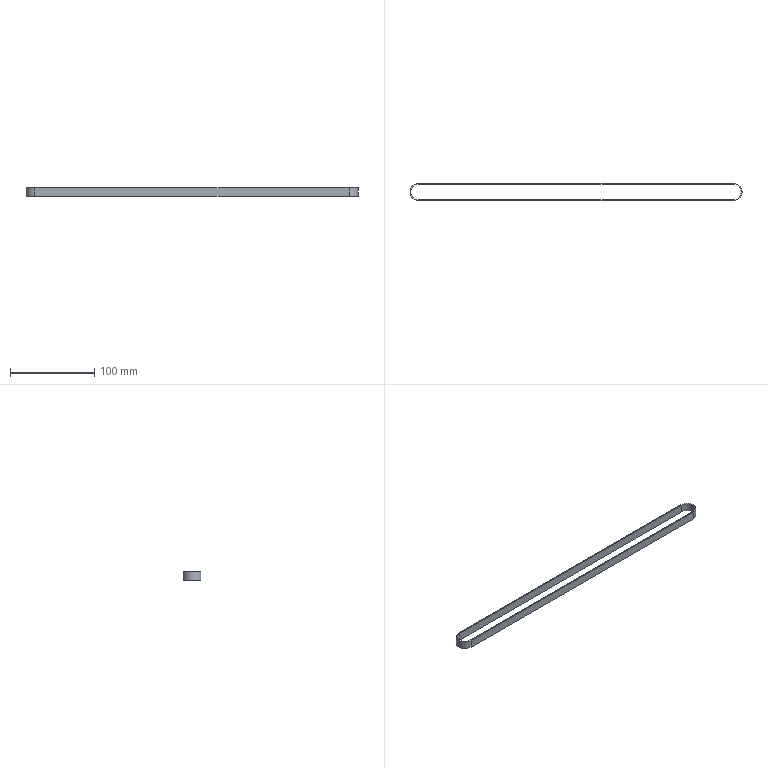Part | SolidWorks | features BaseBody 1 | 1 solid | 12 faces | box 395.01 x 21.01 x 10 mm | volume 8109 mm3 | cylinder 6 | plane 6 | commonest cylinder face diameters 19.01 x3 21.01 x3
STEP:
#1=CARTESIAN_POINT('',(334.,4.505,0.));
#2=VERTEX_POINT('',#1);
#3=CARTESIAN_POINT('',(343.505,-5.,0.));
#4=VERTEX_POINT('',#3);
#5=CARTESIAN_POINT('',(334.,-5.,0.));
#6=DIRECTION('',(0.,0.,-1.));
#7=DIRECTION('',(1.,0.,0.));
#8=AXIS2_PLACEMENT_3D('',#5,#6,#7);
#9=CIRCLE('',#8,9.505);
#10=EDGE_CURVE('',#2,#4,#9,.T.);
#11=ORIENTED_EDGE('',*,*,#10,.T.);
#12=CARTESIAN_POINT('',(343.505,-5.,10.));
#13=VERTEX_POINT('',#12);
#14=CARTESIAN_POINT('',(343.505,-5.,0.));
#15=DIRECTION('',(0.,0.,1.));
#16=VECTOR('',#15,1000.);
#17=LINE('',#14,#16);
#18=EDGE_CURVE('',#4,#13,#17,.T.);
#19=ORIENTED_EDGE('',*,*,#18,.T.);
#20=CARTESIAN_POINT('',(334.,4.505,10.));
#21=VERTEX_POINT('',#20);
#22=CARTESIAN_POINT('',(334.,-5.,10.));
#23=DIRECTION('',(0.,0.,-1.));
#24=DIRECTION('',(1.,0.,0.));
#25=AXIS2_PLACEMENT_3D('',#22,#23,#24);
#26=CIRCLE('',#25,9.505);
#27=EDGE_CURVE('',#21,#13,#26,.T.);
#28=ORIENTED_EDGE('',*,*,#27,.F.);
#29=CARTESIAN_POINT('',(334.,4.505,0.));
#30=DIRECTION('',(0.,0.,-1.));
#31=VECTOR('',#30,1000.);
#32=LINE('',#29,#31);
#33=EDGE_CURVE('',#21,#2,#32,.T.);
#34=ORIENTED_EDGE('',*,*,#33,.T.);
#35=EDGE_LOOP('',(#11,#19,#28,#34));
#36=FACE_OUTER_BOUND('',#35,.T.);
#37=CARTESIAN_POINT('',(334.,-5.,0.));
#38=DIRECTION('',(0.,0.,1.));
#39=DIRECTION('',(1.,0.,0.));
#40=AXIS2_PLACEMENT_3D('',#37,#38,#39);
#41=CYLINDRICAL_SURFACE('',#40,9.505);
#42=ADVANCED_FACE('',(#36),#41,.F.);
#43=CARTESIAN_POINT('',(334.,-15.505,0.));
#44=VERTEX_POINT('',#43);
#45=CARTESIAN_POINT('',(344.505,-5.,0.));
#46=VERTEX_POINT('',#45);
#47=CARTESIAN_POINT('',(334.,-5.,0.));
#48=DIRECTION('',(0.,0.,1.));
#49=DIRECTION('',(1.,0.,0.));
#50=AXIS2_PLACEMENT_3D('',#47,#48,#49);
#51=CIRCLE('',#50,10.505);
#52=EDGE_CURVE('',#44,#46,#51,.T.);
#53=ORIENTED_EDGE('',*,*,#52,.T.);
#54=CARTESIAN_POINT('',(344.505,-5.,10.));
#55=VERTEX_POINT('',#54);
#56=CARTESIAN_POINT('',(344.505,-5.,0.));
#57=DIRECTION('',(0.,0.,1.));
#58=VECTOR('',#57,1000.);
#59=LINE('',#56,#58);
#60=EDGE_CURVE('',#46,#55,#59,.T.);
#61=ORIENTED_EDGE('',*,*,#60,.T.);
#62=CARTESIAN_POINT('',(334.,-15.505,10.));
#63=VERTEX_POINT('',#62);
#64=CARTESIAN_POINT('',(334.,-5.,10.));
#65=DIRECTION('',(0.,0.,1.));
#66=DIRECTION('',(1.,0.,0.));
#67=AXIS2_PLACEMENT_3D('',#64,#65,#66);
#68=CIRCLE('',#67,10.505);
#69=EDGE_CURVE('',#63,#55,#68,.T.);
#70=ORIENTED_EDGE('',*,*,#69,.F.);
#71=CARTESIAN_POINT('',(334.,-15.505,0.));
#72=DIRECTION('',(0.,0.,-1.));
#73=VECTOR('',#72,1000.);
#74=LINE('',#71,#73);
#75=EDGE_CURVE('',#63,#44,#74,.T.);
#76=ORIENTED_EDGE('',*,*,#75,.T.);
#77=EDGE_LOOP('',(#53,#61,#70,#76));
#78=FACE_OUTER_BOUND('',#77,.T.);
#79=CARTESIAN_POINT('',(334.,-5.,0.));
#80=DIRECTION('',(0.,0.,1.));
#81=DIRECTION('',(1.,0.,0.));
#82=AXIS2_PLACEMENT_3D('',#79,#80,#81);
#83=CYLINDRICAL_SURFACE('',#82,10.505);
#84=ADVANCED_FACE('',(#78),#83,.T.);
#85=CARTESIAN_POINT('',(-40.,4.505,0.));
#86=VERTEX_POINT('',#85);
#87=CARTESIAN_POINT('',(-40.,4.505,10.));
#88=VERTEX_POINT('',#87);
#89=CARTESIAN_POINT('',(-40.,4.505,0.));
#90=DIRECTION('',(0.,0.,1.));
#91=VECTOR('',#90,1000.);
#92=LINE('',#89,#91);
#93=EDGE_CURVE('',#86,#88,#92,.T.);
#94=ORIENTED_EDGE('',*,*,#93,.F.);
#95=CARTESIAN_POINT('',(-40.,4.505,0.));
#96=DIRECTION('',(-1.,0.,0.));
#97=VECTOR('',#96,1000.);
#98=LINE('',#95,#97);
#99=EDGE_CURVE('',#2,#86,#98,.T.);
#100=ORIENTED_EDGE('',*,*,#99,.F.);
#101=ORIENTED_EDGE('',*,*,#33,.F.);
#102=CARTESIAN_POINT('',(-40.,4.505,10.));
#103=DIRECTION('',(1.,0.,0.));
#104=VECTOR('',#103,1000.);
#105=LINE('',#102,#104);
#106=EDGE_CURVE('',#88,#21,#105,.T.);
#107=ORIENTED_EDGE('',*,*,#106,.F.);
#108=EDGE_LOOP('',(#94,#100,#101,#107));
#109=FACE_OUTER_BOUND('',#108,.T.);
#110=CARTESIAN_POINT('',(-40.,4.505,0.));
#111=DIRECTION('',(0.,1.,0.));
#112=DIRECTION('',(0.,0.,1.));
#113=AXIS2_PLACEMENT_3D('',#110,#111,#112);
#114=PLANE('',#113);
#115=ADVANCED_FACE('',(#109),#114,.F.);
#116=ORIENTED_EDGE('',*,*,#27,.T.);
#117=CARTESIAN_POINT('',(334.,-14.505,10.));
#118=VERTEX_POINT('',#117);
#119=CARTESIAN_POINT('',(334.,-5.,10.));
#120=DIRECTION('',(0.,0.,-1.));
#121=DIRECTION('',(1.,0.,0.));
#122=AXIS2_PLACEMENT_3D('',#119,#120,#121);
#123=CIRCLE('',#122,9.505);
#124=EDGE_CURVE('',#13,#118,#123,.T.);
#125=ORIENTED_EDGE('',*,*,#124,.T.);
#126=CARTESIAN_POINT('',(-40.,-14.505,10.));
#127=VERTEX_POINT('',#126);
#128=CARTESIAN_POINT('',(147.,-14.505,10.));
#129=DIRECTION('',(-1.,0.,0.));
#130=VECTOR('',#129,1000.);
#131=LINE('',#128,#130);
#132=EDGE_CURVE('',#118,#127,#131,.T.);
#133=ORIENTED_EDGE('',*,*,#132,.T.);
#134=CARTESIAN_POINT('',(-40.,-5.,10.));
#135=DIRECTION('',(0.,0.,-1.));
#136=DIRECTION('',(1.,0.,0.));
#137=AXIS2_PLACEMENT_3D('',#134,#135,#136);
#138=CIRCLE('',#137,9.505);
#139=EDGE_CURVE('',#127,#88,#138,.T.);
#140=ORIENTED_EDGE('',*,*,#139,.T.);
#141=ORIENTED_EDGE('',*,*,#106,.T.);
#142=EDGE_LOOP('',(#116,#125,#133,#140,#141));
#143=FACE_BOUND('',#142,.T.);
#144=ORIENTED_EDGE('',*,*,#69,.T.);
#145=CARTESIAN_POINT('',(334.,5.505,10.));
#146=VERTEX_POINT('',#145);
#147=CARTESIAN_POINT('',(334.,-5.,10.));
#148=DIRECTION('',(0.,0.,1.));
#149=DIRECTION('',(1.,0.,0.));
#150=AXIS2_PLACEMENT_3D('',#147,#148,#149);
#151=CIRCLE('',#150,10.505);
#152=EDGE_CURVE('',#55,#146,#151,.T.);
#153=ORIENTED_EDGE('',*,*,#152,.T.);
#154=CARTESIAN_POINT('',(-40.,5.505,10.));
#155=VERTEX_POINT('',#154);
#156=CARTESIAN_POINT('',(147.,5.505,10.));
#157=DIRECTION('',(-1.,0.,0.));
#158=VECTOR('',#157,1000.);
#159=LINE('',#156,#158);
#160=EDGE_CURVE('',#146,#155,#159,.T.);
#161=ORIENTED_EDGE('',*,*,#160,.T.);
#162=CARTESIAN_POINT('',(-40.,-15.505,10.));
#163=VERTEX_POINT('',#162);
#164=CARTESIAN_POINT('',(-40.,-5.,10.));
#165=DIRECTION('',(0.,0.,1.));
#166=DIRECTION('',(1.,0.,0.));
#167=AXIS2_PLACEMENT_3D('',#164,#165,#166);
#168=CIRCLE('',#167,10.505);
#169=EDGE_CURVE('',#155,#163,#168,.T.);
#170=ORIENTED_EDGE('',*,*,#169,.T.);
#171=CARTESIAN_POINT('',(147.,-15.505,10.));
#172=DIRECTION('',(1.,0.,0.));
#173=VECTOR('',#172,1000.);
#174=LINE('',#171,#173);
#175=EDGE_CURVE('',#163,#63,#174,.T.);
#176=ORIENTED_EDGE('',*,*,#175,.T.);
#177=EDGE_LOOP('',(#144,#153,#161,#170,#176));
#178=FACE_OUTER_BOUND('',#177,.T.);
#179=CARTESIAN_POINT('',(147.,-5.,10.));
#180=DIRECTION('',(0.,0.,1.));
#181=DIRECTION('',(1.,0.,0.));
#182=AXIS2_PLACEMENT_3D('',#179,#180,#181);
#183=PLANE('',#182);
#184=ADVANCED_FACE('',(#143,#178),#183,.T.);
#185=CARTESIAN_POINT('',(-40.,-14.505,0.));
#186=VERTEX_POINT('',#185);
#187=CARTESIAN_POINT('',(-40.,-14.505,0.));
#188=DIRECTION('',(0.,0.,1.));
#189=VECTOR('',#188,1000.);
#190=LINE('',#187,#189);
#191=EDGE_CURVE('',#186,#127,#190,.T.);
#192=ORIENTED_EDGE('',*,*,#191,.F.);
#193=CARTESIAN_POINT('',(-40.,-5.,0.));
#194=DIRECTION('',(0.,0.,1.));
#195=DIRECTION('',(1.,0.,0.));
#196=AXIS2_PLACEMENT_3D('',#193,#194,#195);
#197=CIRCLE('',#196,9.505);
#198=EDGE_CURVE('',#86,#186,#197,.T.);
#199=ORIENTED_EDGE('',*,*,#198,.F.);
#200=ORIENTED_EDGE('',*,*,#93,.T.);
#201=ORIENTED_EDGE('',*,*,#139,.F.);
#202=EDGE_LOOP('',(#192,#199,#200,#201));
#203=FACE_OUTER_BOUND('',#202,.T.);
#204=CARTESIAN_POINT('',(-40.,-5.,0.));
#205=DIRECTION('',(0.,0.,1.));
#206=DIRECTION('',(1.,0.,0.));
#207=AXIS2_PLACEMENT_3D('',#204,#205,#206);
#208=CYLINDRICAL_SURFACE('',#207,9.505);
#209=ADVANCED_FACE('',(#203),#208,.F.);
#210=CARTESIAN_POINT('',(334.,-14.505,0.));
#211=VERTEX_POINT('',#210);
#212=CARTESIAN_POINT('',(147.,-14.505,0.));
#213=DIRECTION('',(-1.,0.,0.));
#214=VECTOR('',#213,1000.);
#215=LINE('',#212,#214);
#216=EDGE_CURVE('',#211,#186,#215,.T.);
#217=ORIENTED_EDGE('',*,*,#216,.F.);
#218=CARTESIAN_POINT('',(334.,-5.,0.));
#219=DIRECTION('',(0.,0.,-1.));
#220=DIRECTION('',(1.,0.,0.));
#221=AXIS2_PLACEMENT_3D('',#218,#219,#220);
#222=CIRCLE('',#221,9.505);
#223=EDGE_CURVE('',#4,#211,#222,.T.);
#224=ORIENTED_EDGE('',*,*,#223,.F.);
#225=ORIENTED_EDGE('',*,*,#10,.F.);
#226=ORIENTED_EDGE('',*,*,#99,.T.);
#227=ORIENTED_EDGE('',*,*,#198,.T.);
#228=EDGE_LOOP('',(#217,#224,#225,#226,#227));
#229=FACE_BOUND('',#228,.T.);
#230=CARTESIAN_POINT('',(-40.,5.505,0.));
#231=VERTEX_POINT('',#230);
#232=CARTESIAN_POINT('',(-40.,-15.505,0.));
#233=VERTEX_POINT('',#232);
#234=CARTESIAN_POINT('',(-40.,-5.,0.));
#235=DIRECTION('',(0.,0.,1.));
#236=DIRECTION('',(1.,0.,0.));
#237=AXIS2_PLACEMENT_3D('',#234,#235,#236);
#238=CIRCLE('',#237,10.505);
#239=EDGE_CURVE('',#231,#233,#238,.T.);
#240=ORIENTED_EDGE('',*,*,#239,.F.);
#241=CARTESIAN_POINT('',(334.,5.505,0.));
#242=VERTEX_POINT('',#241);
#243=CARTESIAN_POINT('',(147.,5.505,0.));
#244=DIRECTION('',(-1.,0.,0.));
#245=VECTOR('',#244,1000.);
#246=LINE('',#243,#245);
#247=EDGE_CURVE('',#242,#231,#246,.T.);
#248=ORIENTED_EDGE('',*,*,#247,.F.);
#249=CARTESIAN_POINT('',(334.,-5.,0.));
#250=DIRECTION('',(0.,0.,1.));
#251=DIRECTION('',(1.,0.,0.));
#252=AXIS2_PLACEMENT_3D('',#249,#250,#251);
#253=CIRCLE('',#252,10.505);
#254=EDGE_CURVE('',#46,#242,#253,.T.);
#255=ORIENTED_EDGE('',*,*,#254,.F.);
#256=ORIENTED_EDGE('',*,*,#52,.F.);
#257=CARTESIAN_POINT('',(147.,-15.505,0.));
#258=DIRECTION('',(1.,0.,0.));
#259=VECTOR('',#258,1000.);
#260=LINE('',#257,#259);
#261=EDGE_CURVE('',#233,#44,#260,.T.);
#262=ORIENTED_EDGE('',*,*,#261,.F.);
#263=EDGE_LOOP('',(#240,#248,#255,#256,#262));
#264=FACE_OUTER_BOUND('',#263,.T.);
#265=CARTESIAN_POINT('',(147.,-5.,0.));
#266=DIRECTION('',(0.,0.,1.));
#267=DIRECTION('',(1.,0.,0.));
#268=AXIS2_PLACEMENT_3D('',#265,#266,#267);
#269=PLANE('',#268);
#270=ADVANCED_FACE('',(#229,#264),#269,.F.);
#271=ORIENTED_EDGE('',*,*,#18,.F.);
#272=ORIENTED_EDGE('',*,*,#223,.T.);
#273=CARTESIAN_POINT('',(334.,-14.505,0.));
#274=DIRECTION('',(0.,0.,-1.));
#275=VECTOR('',#274,1000.);
#276=LINE('',#273,#275);
#277=EDGE_CURVE('',#118,#211,#276,.T.);
#278=ORIENTED_EDGE('',*,*,#277,.F.);
#279=ORIENTED_EDGE('',*,*,#124,.F.);
#280=EDGE_LOOP('',(#271,#272,#278,#279));
#281=FACE_OUTER_BOUND('',#280,.T.);
#282=CARTESIAN_POINT('',(334.,-5.,0.));
#283=DIRECTION('',(0.,0.,1.));
#284=DIRECTION('',(1.,0.,0.));
#285=AXIS2_PLACEMENT_3D('',#282,#283,#284);
#286=CYLINDRICAL_SURFACE('',#285,9.505);
#287=ADVANCED_FACE('',(#281),#286,.F.);
#288=ORIENTED_EDGE('',*,*,#277,.T.);
#289=ORIENTED_EDGE('',*,*,#216,.T.);
#290=ORIENTED_EDGE('',*,*,#191,.T.);
#291=ORIENTED_EDGE('',*,*,#132,.F.);
#292=EDGE_LOOP('',(#288,#289,#290,#291));
#293=FACE_OUTER_BOUND('',#292,.T.);
#294=CARTESIAN_POINT('',(334.,-14.505,0.));
#295=DIRECTION('',(0.,-1.,0.));
#296=DIRECTION('',(0.,0.,-1.));
#297=AXIS2_PLACEMENT_3D('',#294,#295,#296);
#298=PLANE('',#297);
#299=ADVANCED_FACE('',(#293),#298,.F.);
#300=ORIENTED_EDGE('',*,*,#247,.T.);
#301=CARTESIAN_POINT('',(-40.,5.505,0.));
#302=DIRECTION('',(0.,0.,1.));
#303=VECTOR('',#302,1000.);
#304=LINE('',#301,#303);
#305=EDGE_CURVE('',#231,#155,#304,.T.);
#306=ORIENTED_EDGE('',*,*,#305,.T.);
#307=ORIENTED_EDGE('',*,*,#160,.F.);
#308=CARTESIAN_POINT('',(334.,5.505,0.));
#309=DIRECTION('',(0.,0.,-1.));
#310=VECTOR('',#309,1000.);
#311=LINE('',#308,#310);
#312=EDGE_CURVE('',#146,#242,#311,.T.);
#313=ORIENTED_EDGE('',*,*,#312,.T.);
#314=EDGE_LOOP('',(#300,#306,#307,#313));
#315=FACE_OUTER_BOUND('',#314,.T.);
#316=CARTESIAN_POINT('',(-40.,5.505,0.));
#317=DIRECTION('',(0.,1.,0.));
#318=DIRECTION('',(0.,0.,1.));
#319=AXIS2_PLACEMENT_3D('',#316,#317,#318);
#320=PLANE('',#319);
#321=ADVANCED_FACE('',(#315),#320,.T.);
#322=ORIENTED_EDGE('',*,*,#60,.F.);
#323=ORIENTED_EDGE('',*,*,#254,.T.);
#324=ORIENTED_EDGE('',*,*,#312,.F.);
#325=ORIENTED_EDGE('',*,*,#152,.F.);
#326=EDGE_LOOP('',(#322,#323,#324,#325));
#327=FACE_OUTER_BOUND('',#326,.T.);
#328=CARTESIAN_POINT('',(334.,-5.,0.));
#329=DIRECTION('',(0.,0.,1.));
#330=DIRECTION('',(1.,0.,0.));
#331=AXIS2_PLACEMENT_3D('',#328,#329,#330);
#332=CYLINDRICAL_SURFACE('',#331,10.505);
#333=ADVANCED_FACE('',(#327),#332,.T.);
#334=ORIENTED_EDGE('',*,*,#261,.T.);
#335=ORIENTED_EDGE('',*,*,#75,.F.);
#336=ORIENTED_EDGE('',*,*,#175,.F.);
#337=CARTESIAN_POINT('',(-40.,-15.505,0.));
#338=DIRECTION('',(0.,0.,-1.));
#339=VECTOR('',#338,1000.);
#340=LINE('',#337,#339);
#341=EDGE_CURVE('',#163,#233,#340,.T.);
#342=ORIENTED_EDGE('',*,*,#341,.T.);
#343=EDGE_LOOP('',(#334,#335,#336,#342));
#344=FACE_OUTER_BOUND('',#343,.T.);
#345=CARTESIAN_POINT('',(334.,-15.505,0.));
#346=DIRECTION('',(0.,-1.,0.));
#347=DIRECTION('',(0.,0.,-1.));
#348=AXIS2_PLACEMENT_3D('',#345,#346,#347);
#349=PLANE('',#348);
#350=ADVANCED_FACE('',(#344),#349,.T.);
#351=ORIENTED_EDGE('',*,*,#239,.T.);
#352=ORIENTED_EDGE('',*,*,#341,.F.);
#353=ORIENTED_EDGE('',*,*,#169,.F.);
#354=ORIENTED_EDGE('',*,*,#305,.F.);
#355=EDGE_LOOP('',(#351,#352,#353,#354));
#356=FACE_OUTER_BOUND('',#355,.T.);
#357=CARTESIAN_POINT('',(-40.,-5.,0.));
#358=DIRECTION('',(0.,0.,1.));
#359=DIRECTION('',(1.,0.,0.));
#360=AXIS2_PLACEMENT_3D('',#357,#358,#359);
#361=CYLINDRICAL_SURFACE('',#360,10.505);
#362=ADVANCED_FACE('',(#356),#361,.T.);
#363=CLOSED_SHELL('',(#42,#84,#115,#184,#209,#270,#287,#299,#321,#333,#350,#362));
#364=MANIFOLD_SOLID_BREP('',#363);
#365=CARTESIAN_POINT('',(0.,0.,0.));
#366=DIRECTION('',(0.,0.,1.));
#367=DIRECTION('',(1.,0.,0.));
#368=AXIS2_PLACEMENT_3D('',#365,#366,#367);
#369=(LENGTH_UNIT()NAMED_UNIT(*)SI_UNIT(.MILLI.,.METRE.));
#370=UNCERTAINTY_MEASURE_WITH_UNIT(LENGTH_MEASURE(0.00001),#369,'','');
#371=(NAMED_UNIT(*)PLANE_ANGLE_UNIT()SI_UNIT($,.RADIAN.));
#372=(NAMED_UNIT(*)SI_UNIT($,.STERADIAN.)SOLID_ANGLE_UNIT());
#373=(GEOMETRIC_REPRESENTATION_CONTEXT(3)GLOBAL_UNCERTAINTY_ASSIGNED_CONTEXT((#370))GLOBAL_UNIT_ASSIGNED_CONTEXT((#369,#371,#372))REPRESENTATION_CONTEXT('',''));
#374=ADVANCED_BREP_SHAPE_REPRESENTATION('',(#364,#368),#373);